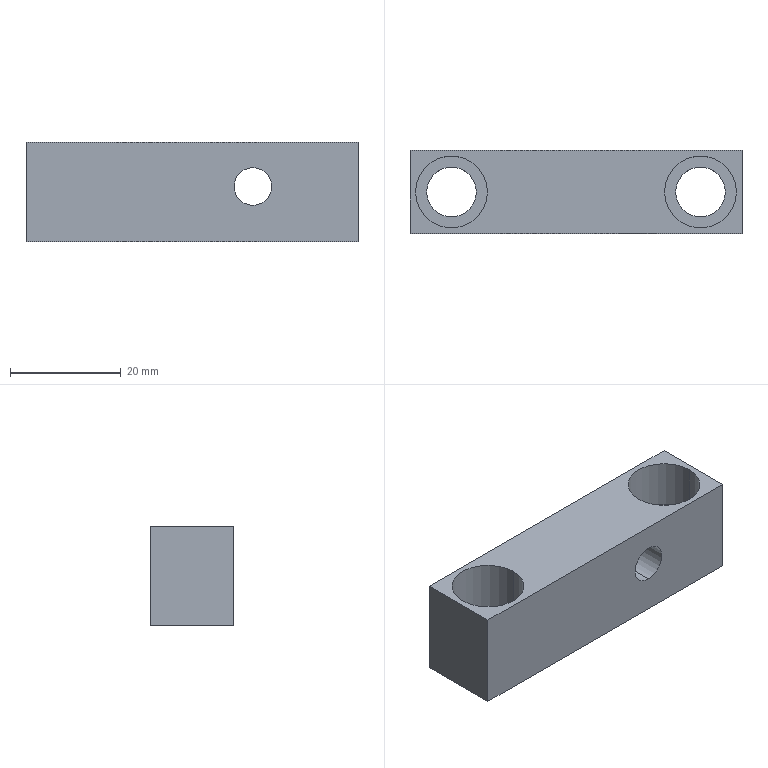Part | STEP file | Tensioning part | 1 solid | 18 faces | box 60 x 15 x 18 mm | volume 12121 mm3 | cylinder 10 | plane 8 | commonest cylinder face diameters 9 x4 13 x4 6.8 x2
STEP:
#1=CARTESIAN_POINT('',(0.,0.,0.));
#2=DIRECTION('',(0.,0.,1.));
#3=DIRECTION('',(1.,0.,0.));
#4=AXIS2_PLACEMENT_3D('',#1,#2,#3);
#5=CARTESIAN_POINT('',(11.,-7.5,13.4));
#6=VERTEX_POINT('',#5);
#7=CARTESIAN_POINT('',(11.,7.5,13.4));
#8=VERTEX_POINT('',#7);
#9=CARTESIAN_POINT('',(11.,7.5,13.4));
#10=DIRECTION('',(0.,1.,0.));
#11=VECTOR('',#10,1.);
#12=LINE('',#9,#11);
#13=CARTESIAN_POINT('',(11.,7.5,10.));
#14=DIRECTION('',(0.,1.,0.));
#15=DIRECTION('',(0.,0.,1.));
#16=AXIS2_PLACEMENT_3D('',#13,#14,#15);
#17=CYLINDRICAL_SURFACE('',#16,3.4);
#18=CARTESIAN_POINT('',(6.283,0.));
#19=DIRECTION('',(0.,1.));
#20=VECTOR('',#19,1.);
#21=LINE('',#18,#20);
#22=(GEOMETRIC_REPRESENTATION_CONTEXT(2)PARAMETRIC_REPRESENTATION_CONTEXT()REPRESENTATION_CONTEXT('',''));
#23=DEFINITIONAL_REPRESENTATION('',(#21),#22);
#24=PCURVE('',#17,#23);
#25=CARTESIAN_POINT('',(11.,7.5,10.));
#26=DIRECTION('',(0.,1.,0.));
#27=DIRECTION('',(0.,0.,1.));
#28=AXIS2_PLACEMENT_3D('',#25,#26,#27);
#29=CYLINDRICAL_SURFACE('',#28,3.4);
#30=CARTESIAN_POINT('',(0.,0.));
#31=DIRECTION('',(0.,1.));
#32=VECTOR('',#31,1.);
#33=LINE('',#30,#32);
#34=(GEOMETRIC_REPRESENTATION_CONTEXT(2)PARAMETRIC_REPRESENTATION_CONTEXT()REPRESENTATION_CONTEXT('',''));
#35=DEFINITIONAL_REPRESENTATION('',(#33),#34);
#36=PCURVE('',#29,#35);
#37=SURFACE_CURVE('',#12,(#24,#36),.PCURVE_S1.);
#38=EDGE_CURVE('',#6,#8,#37,.T.);
#39=ORIENTED_EDGE('',*,*,#38,.T.);
#40=CARTESIAN_POINT('',(11.,7.5,6.6));
#41=VERTEX_POINT('',#40);
#42=CARTESIAN_POINT('',(11.,7.5,10.));
#43=DIRECTION('',(0.,1.,0.));
#44=DIRECTION('',(0.,0.,1.));
#45=AXIS2_PLACEMENT_3D('',#42,#43,#44);
#46=CIRCLE('',#45,3.4);
#47=CARTESIAN_POINT('',(0.,0.));
#48=DIRECTION('',(1.,0.));
#49=VECTOR('',#48,1.);
#50=LINE('',#47,#49);
#51=(GEOMETRIC_REPRESENTATION_CONTEXT(2)PARAMETRIC_REPRESENTATION_CONTEXT()REPRESENTATION_CONTEXT('',''));
#52=DEFINITIONAL_REPRESENTATION('',(#50),#51);
#53=PCURVE('',#17,#52);
#54=CARTESIAN_POINT('',(-30.,7.5,18.));
#55=DIRECTION('',(0.,-1.,0.));
#56=DIRECTION('',(0.,0.,-1.));
#57=AXIS2_PLACEMENT_3D('',#54,#55,#56);
#58=PLANE('',#57);
#59=CARTESIAN_POINT('',(4.6,41.));
#60=CARTESIAN_POINT('',(4.6,46.889));
#61=CARTESIAN_POINT('',(9.7,43.944));
#62=CARTESIAN_POINT('',(14.8,41.));
#63=CARTESIAN_POINT('',(9.7,38.056));
#64=CARTESIAN_POINT('',(4.6,35.111));
#65=CARTESIAN_POINT('',(4.6,41.));
#66=(BOUNDED_CURVE()B_SPLINE_CURVE(2,(#59,#60,#61,#62,#63,#64,#65),.UNSPECIFIED.,.T.,.F.)B_SPLINE_CURVE_WITH_KNOTS((1,2,2,2,2,1),(-2.094,0.,2.094,4.189,6.283,8.378),.UNSPECIFIED.)CURVE()GEOMETRIC_REPRESENTATION_ITEM()RATIONAL_B_SPLINE_CURVE((1.,0.5,1.,0.5,1.,0.5,1.))REPRESENTATION_ITEM(''));
#67=(GEOMETRIC_REPRESENTATION_CONTEXT(2)PARAMETRIC_REPRESENTATION_CONTEXT()REPRESENTATION_CONTEXT('',''));
#68=DEFINITIONAL_REPRESENTATION('',(#66),#67);
#69=PCURVE('',#58,#68);
#70=SURFACE_CURVE('',#46,(#53,#69),.PCURVE_S1.);
#71=EDGE_CURVE('',#41,#8,#70,.T.);
#72=ORIENTED_EDGE('',*,*,#71,.F.);
#73=CARTESIAN_POINT('',(11.,-7.5,6.6));
#74=VERTEX_POINT('',#73);
#75=CARTESIAN_POINT('',(11.,7.5,6.6));
#76=DIRECTION('',(0.,1.,0.));
#77=VECTOR('',#76,1.);
#78=LINE('',#75,#77);
#79=CARTESIAN_POINT('',(3.142,0.));
#80=DIRECTION('',(0.,1.));
#81=VECTOR('',#80,1.);
#82=LINE('',#79,#81);
#83=(GEOMETRIC_REPRESENTATION_CONTEXT(2)PARAMETRIC_REPRESENTATION_CONTEXT()REPRESENTATION_CONTEXT('',''));
#84=DEFINITIONAL_REPRESENTATION('',(#82),#83);
#85=PCURVE('',#17,#84);
#86=CARTESIAN_POINT('',(3.142,0.));
#87=DIRECTION('',(0.,1.));
#88=VECTOR('',#87,1.);
#89=LINE('',#86,#88);
#90=(GEOMETRIC_REPRESENTATION_CONTEXT(2)PARAMETRIC_REPRESENTATION_CONTEXT()REPRESENTATION_CONTEXT('',''));
#91=DEFINITIONAL_REPRESENTATION('',(#89),#90);
#92=PCURVE('',#29,#91);
#93=SURFACE_CURVE('',#78,(#85,#92),.PCURVE_S1.);
#94=EDGE_CURVE('',#74,#41,#93,.T.);
#95=ORIENTED_EDGE('',*,*,#94,.F.);
#96=CARTESIAN_POINT('',(11.,-7.5,10.));
#97=DIRECTION('',(0.,1.,0.));
#98=DIRECTION('',(0.,0.,1.));
#99=AXIS2_PLACEMENT_3D('',#96,#97,#98);
#100=CIRCLE('',#99,3.4);
#101=CARTESIAN_POINT('',(0.,-15.));
#102=DIRECTION('',(1.,0.));
#103=VECTOR('',#102,1.);
#104=LINE('',#101,#103);
#105=(GEOMETRIC_REPRESENTATION_CONTEXT(2)PARAMETRIC_REPRESENTATION_CONTEXT()REPRESENTATION_CONTEXT('',''));
#106=DEFINITIONAL_REPRESENTATION('',(#104),#105);
#107=PCURVE('',#17,#106);
#108=CARTESIAN_POINT('',(-30.,-7.5,18.));
#109=DIRECTION('',(0.,1.,0.));
#110=DIRECTION('',(0.,0.,1.));
#111=AXIS2_PLACEMENT_3D('',#108,#109,#110);
#112=PLANE('',#111);
#113=CARTESIAN_POINT('',(-8.,41.));
#114=DIRECTION('',(1.,0.));
#115=AXIS2_PLACEMENT_2D('',#113,#114);
#116=CIRCLE('',#115,3.4);
#117=(GEOMETRIC_REPRESENTATION_CONTEXT(2)PARAMETRIC_REPRESENTATION_CONTEXT()REPRESENTATION_CONTEXT('',''));
#118=DEFINITIONAL_REPRESENTATION('',(#116),#117);
#119=PCURVE('',#112,#118);
#120=SURFACE_CURVE('',#100,(#107,#119),.PCURVE_S1.);
#121=EDGE_CURVE('',#74,#6,#120,.T.);
#122=ORIENTED_EDGE('',*,*,#121,.T.);
#123=EDGE_LOOP('',(#39,#72,#95,#122));
#124=FACE_BOUND('',#123,.F.);
#125=ADVANCED_FACE('',(#124),#17,.F.);
#126=CARTESIAN_POINT('',(-16.,0.,9.));
#127=VERTEX_POINT('',#126);
#128=CARTESIAN_POINT('',(-16.,0.,18.));
#129=VERTEX_POINT('',#128);
#130=CARTESIAN_POINT('',(-16.,0.,18.));
#131=DIRECTION('',(0.,0.,1.));
#132=VECTOR('',#131,1.);
#133=LINE('',#130,#132);
#134=CARTESIAN_POINT('',(-22.5,0.,18.));
#135=DIRECTION('',(0.,0.,1.));
#136=DIRECTION('',(1.,0.,0.));
#137=AXIS2_PLACEMENT_3D('',#134,#135,#136);
#138=CYLINDRICAL_SURFACE('',#137,6.5);
#139=CARTESIAN_POINT('',(6.283,0.));
#140=DIRECTION('',(0.,1.));
#141=VECTOR('',#140,1.);
#142=LINE('',#139,#141);
#143=(GEOMETRIC_REPRESENTATION_CONTEXT(2)PARAMETRIC_REPRESENTATION_CONTEXT()REPRESENTATION_CONTEXT('',''));
#144=DEFINITIONAL_REPRESENTATION('',(#142),#143);
#145=PCURVE('',#138,#144);
#146=CARTESIAN_POINT('',(-22.5,0.,18.));
#147=DIRECTION('',(0.,0.,1.));
#148=DIRECTION('',(1.,0.,0.));
#149=AXIS2_PLACEMENT_3D('',#146,#147,#148);
#150=CYLINDRICAL_SURFACE('',#149,6.5);
#151=CARTESIAN_POINT('',(0.,0.));
#152=DIRECTION('',(0.,1.));
#153=VECTOR('',#152,1.);
#154=LINE('',#151,#153);
#155=(GEOMETRIC_REPRESENTATION_CONTEXT(2)PARAMETRIC_REPRESENTATION_CONTEXT()REPRESENTATION_CONTEXT('',''));
#156=DEFINITIONAL_REPRESENTATION('',(#154),#155);
#157=PCURVE('',#150,#156);
#158=SURFACE_CURVE('',#133,(#145,#157),.PCURVE_S1.);
#159=EDGE_CURVE('',#127,#129,#158,.T.);
#160=ORIENTED_EDGE('',*,*,#159,.T.);
#161=CARTESIAN_POINT('',(-29.,0.,18.));
#162=VERTEX_POINT('',#161);
#163=CARTESIAN_POINT('',(-22.5,0.,18.));
#164=DIRECTION('',(0.,0.,1.));
#165=DIRECTION('',(1.,0.,0.));
#166=AXIS2_PLACEMENT_3D('',#163,#164,#165);
#167=CIRCLE('',#166,6.5);
#168=CARTESIAN_POINT('',(0.,0.));
#169=DIRECTION('',(1.,0.));
#170=VECTOR('',#169,1.);
#171=LINE('',#168,#170);
#172=(GEOMETRIC_REPRESENTATION_CONTEXT(2)PARAMETRIC_REPRESENTATION_CONTEXT()REPRESENTATION_CONTEXT('',''));
#173=DEFINITIONAL_REPRESENTATION('',(#171),#172);
#174=PCURVE('',#138,#173);
#175=CARTESIAN_POINT('',(0.,0.,18.));
#176=DIRECTION('',(0.,0.,1.));
#177=DIRECTION('',(1.,0.,0.));
#178=AXIS2_PLACEMENT_3D('',#175,#176,#177);
#179=PLANE('',#178);
#180=CARTESIAN_POINT('',(-22.5,0.));
#181=DIRECTION('',(1.,0.));
#182=AXIS2_PLACEMENT_2D('',#180,#181);
#183=CIRCLE('',#182,6.5);
#184=(GEOMETRIC_REPRESENTATION_CONTEXT(2)PARAMETRIC_REPRESENTATION_CONTEXT()REPRESENTATION_CONTEXT('',''));
#185=DEFINITIONAL_REPRESENTATION('',(#183),#184);
#186=PCURVE('',#179,#185);
#187=SURFACE_CURVE('',#167,(#174,#186),.PCURVE_S1.);
#188=EDGE_CURVE('',#162,#129,#187,.T.);
#189=ORIENTED_EDGE('',*,*,#188,.F.);
#190=CARTESIAN_POINT('',(-29.,0.,9.));
#191=VERTEX_POINT('',#190);
#192=CARTESIAN_POINT('',(-29.,0.,18.));
#193=DIRECTION('',(0.,0.,1.));
#194=VECTOR('',#193,1.);
#195=LINE('',#192,#194);
#196=CARTESIAN_POINT('',(3.142,0.));
#197=DIRECTION('',(0.,1.));
#198=VECTOR('',#197,1.);
#199=LINE('',#196,#198);
#200=(GEOMETRIC_REPRESENTATION_CONTEXT(2)PARAMETRIC_REPRESENTATION_CONTEXT()REPRESENTATION_CONTEXT('',''));
#201=DEFINITIONAL_REPRESENTATION('',(#199),#200);
#202=PCURVE('',#138,#201);
#203=CARTESIAN_POINT('',(3.142,0.));
#204=DIRECTION('',(0.,1.));
#205=VECTOR('',#204,1.);
#206=LINE('',#203,#205);
#207=(GEOMETRIC_REPRESENTATION_CONTEXT(2)PARAMETRIC_REPRESENTATION_CONTEXT()REPRESENTATION_CONTEXT('',''));
#208=DEFINITIONAL_REPRESENTATION('',(#206),#207);
#209=PCURVE('',#150,#208);
#210=SURFACE_CURVE('',#195,(#202,#209),.PCURVE_S1.);
#211=EDGE_CURVE('',#191,#162,#210,.T.);
#212=ORIENTED_EDGE('',*,*,#211,.F.);
#213=CARTESIAN_POINT('',(-22.5,0.,9.));
#214=DIRECTION('',(0.,0.,1.));
#215=DIRECTION('',(1.,0.,0.));
#216=AXIS2_PLACEMENT_3D('',#213,#214,#215);
#217=CIRCLE('',#216,6.5);
#218=CARTESIAN_POINT('',(0.,-9.));
#219=DIRECTION('',(1.,0.));
#220=VECTOR('',#219,1.);
#221=LINE('',#218,#220);
#222=(GEOMETRIC_REPRESENTATION_CONTEXT(2)PARAMETRIC_REPRESENTATION_CONTEXT()REPRESENTATION_CONTEXT('',''));
#223=DEFINITIONAL_REPRESENTATION('',(#221),#222);
#224=PCURVE('',#138,#223);
#225=CARTESIAN_POINT('',(-18.,0.,9.));
#226=DIRECTION('',(0.,0.,-1.));
#227=DIRECTION('',(-1.,0.,0.));
#228=AXIS2_PLACEMENT_3D('',#225,#226,#227);
#229=PLANE('',#228);
#230=CARTESIAN_POINT('',(-2.,0.));
#231=CARTESIAN_POINT('',(-2.,11.258));
#232=CARTESIAN_POINT('',(7.75,5.629));
#233=CARTESIAN_POINT('',(17.5,0.));
#234=CARTESIAN_POINT('',(7.75,-5.629));
#235=CARTESIAN_POINT('',(-2.,-11.258));
#236=CARTESIAN_POINT('',(-2.,0.));
#237=(BOUNDED_CURVE()B_SPLINE_CURVE(2,(#230,#231,#232,#233,#234,#235,#236),.UNSPECIFIED.,.T.,.F.)B_SPLINE_CURVE_WITH_KNOTS((1,2,2,2,2,1),(-2.094,0.,2.094,4.189,6.283,8.378),.UNSPECIFIED.)CURVE()GEOMETRIC_REPRESENTATION_ITEM()RATIONAL_B_SPLINE_CURVE((1.,0.5,1.,0.5,1.,0.5,1.))REPRESENTATION_ITEM(''));
#238=(GEOMETRIC_REPRESENTATION_CONTEXT(2)PARAMETRIC_REPRESENTATION_CONTEXT()REPRESENTATION_CONTEXT('',''));
#239=DEFINITIONAL_REPRESENTATION('',(#237),#238);
#240=PCURVE('',#229,#239);
#241=SURFACE_CURVE('',#217,(#224,#240),.PCURVE_S1.);
#242=EDGE_CURVE('',#191,#127,#241,.T.);
#243=ORIENTED_EDGE('',*,*,#242,.T.);
#244=EDGE_LOOP('',(#160,#189,#212,#243));
#245=FACE_BOUND('',#244,.F.);
#246=ADVANCED_FACE('',(#245),#138,.F.);
#247=CARTESIAN_POINT('',(-18.,0.,0.));
#248=VERTEX_POINT('',#247);
#249=CARTESIAN_POINT('',(-18.,0.,9.));
#250=VERTEX_POINT('',#249);
#251=CARTESIAN_POINT('',(-18.,0.,18.));
#252=DIRECTION('',(0.,0.,1.));
#253=VECTOR('',#252,1.);
#254=LINE('',#251,#253);
#255=CARTESIAN_POINT('',(-22.5,0.,18.));
#256=DIRECTION('',(0.,0.,1.));
#257=DIRECTION('',(1.,0.,0.));
#258=AXIS2_PLACEMENT_3D('',#255,#256,#257);
#259=CYLINDRICAL_SURFACE('',#258,4.5);
#260=CARTESIAN_POINT('',(6.283,0.));
#261=DIRECTION('',(0.,1.));
#262=VECTOR('',#261,1.);
#263=LINE('',#260,#262);
#264=(GEOMETRIC_REPRESENTATION_CONTEXT(2)PARAMETRIC_REPRESENTATION_CONTEXT()REPRESENTATION_CONTEXT('',''));
#265=DEFINITIONAL_REPRESENTATION('',(#263),#264);
#266=PCURVE('',#259,#265);
#267=CARTESIAN_POINT('',(-22.5,0.,18.));
#268=DIRECTION('',(0.,0.,1.));
#269=DIRECTION('',(1.,0.,0.));
#270=AXIS2_PLACEMENT_3D('',#267,#268,#269);
#271=CYLINDRICAL_SURFACE('',#270,4.5);
#272=CARTESIAN_POINT('',(0.,0.));
#273=DIRECTION('',(0.,1.));
#274=VECTOR('',#273,1.);
#275=LINE('',#272,#274);
#276=(GEOMETRIC_REPRESENTATION_CONTEXT(2)PARAMETRIC_REPRESENTATION_CONTEXT()REPRESENTATION_CONTEXT('',''));
#277=DEFINITIONAL_REPRESENTATION('',(#275),#276);
#278=PCURVE('',#271,#277);
#279=SURFACE_CURVE('',#254,(#266,#278),.PCURVE_S1.);
#280=EDGE_CURVE('',#248,#250,#279,.T.);
#281=ORIENTED_EDGE('',*,*,#280,.T.);
#282=CARTESIAN_POINT('',(-27.,0.,9.));
#283=VERTEX_POINT('',#282);
#284=CARTESIAN_POINT('',(-22.5,0.,9.));
#285=DIRECTION('',(0.,0.,1.));
#286=DIRECTION('',(1.,0.,0.));
#287=AXIS2_PLACEMENT_3D('',#284,#285,#286);
#288=CIRCLE('',#287,4.5);
#289=CARTESIAN_POINT('',(0.,-9.));
#290=DIRECTION('',(1.,0.));
#291=VECTOR('',#290,1.);
#292=LINE('',#289,#291);
#293=(GEOMETRIC_REPRESENTATION_CONTEXT(2)PARAMETRIC_REPRESENTATION_CONTEXT()REPRESENTATION_CONTEXT('',''));
#294=DEFINITIONAL_REPRESENTATION('',(#292),#293);
#295=PCURVE('',#259,#294);
#296=CARTESIAN_POINT('',(0.,0.));
#297=CARTESIAN_POINT('',(0.,7.794));
#298=CARTESIAN_POINT('',(6.75,3.897));
#299=CARTESIAN_POINT('',(13.5,0.));
#300=CARTESIAN_POINT('',(6.75,-3.897));
#301=CARTESIAN_POINT('',(0.,-7.794));
#302=CARTESIAN_POINT('',(0.,0.));
#303=(BOUNDED_CURVE()B_SPLINE_CURVE(2,(#296,#297,#298,#299,#300,#301,#302),.UNSPECIFIED.,.T.,.F.)B_SPLINE_CURVE_WITH_KNOTS((1,2,2,2,2,1),(-2.094,0.,2.094,4.189,6.283,8.378),.UNSPECIFIED.)CURVE()GEOMETRIC_REPRESENTATION_ITEM()RATIONAL_B_SPLINE_CURVE((1.,0.5,1.,0.5,1.,0.5,1.))REPRESENTATION_ITEM(''));
#304=(GEOMETRIC_REPRESENTATION_CONTEXT(2)PARAMETRIC_REPRESENTATION_CONTEXT()REPRESENTATION_CONTEXT('',''));
#305=DEFINITIONAL_REPRESENTATION('',(#303),#304);
#306=PCURVE('',#229,#305);
#307=SURFACE_CURVE('',#288,(#295,#306),.PCURVE_S1.);
#308=EDGE_CURVE('',#283,#250,#307,.T.);
#309=ORIENTED_EDGE('',*,*,#308,.F.);
#310=CARTESIAN_POINT('',(-27.,0.,0.));
#311=VERTEX_POINT('',#310);
#312=CARTESIAN_POINT('',(-27.,0.,18.));
#313=DIRECTION('',(0.,0.,1.));
#314=VECTOR('',#313,1.);
#315=LINE('',#312,#314);
#316=CARTESIAN_POINT('',(3.142,0.));
#317=DIRECTION('',(0.,1.));
#318=VECTOR('',#317,1.);
#319=LINE('',#316,#318);
#320=(GEOMETRIC_REPRESENTATION_CONTEXT(2)PARAMETRIC_REPRESENTATION_CONTEXT()REPRESENTATION_CONTEXT('',''));
#321=DEFINITIONAL_REPRESENTATION('',(#319),#320);
#322=PCURVE('',#259,#321);
#323=CARTESIAN_POINT('',(3.142,0.));
#324=DIRECTION('',(0.,1.));
#325=VECTOR('',#324,1.);
#326=LINE('',#323,#325);
#327=(GEOMETRIC_REPRESENTATION_CONTEXT(2)PARAMETRIC_REPRESENTATION_CONTEXT()REPRESENTATION_CONTEXT('',''));
#328=DEFINITIONAL_REPRESENTATION('',(#326),#327);
#329=PCURVE('',#271,#328);
#330=SURFACE_CURVE('',#315,(#322,#329),.PCURVE_S1.);
#331=EDGE_CURVE('',#311,#283,#330,.T.);
#332=ORIENTED_EDGE('',*,*,#331,.F.);
#333=CARTESIAN_POINT('',(-22.5,0.,0.));
#334=DIRECTION('',(0.,0.,1.));
#335=DIRECTION('',(1.,0.,0.));
#336=AXIS2_PLACEMENT_3D('',#333,#334,#335);
#337=CIRCLE('',#336,4.5);
#338=CARTESIAN_POINT('',(0.,-18.));
#339=DIRECTION('',(1.,0.));
#340=VECTOR('',#339,1.);
#341=LINE('',#338,#340);
#342=(GEOMETRIC_REPRESENTATION_CONTEXT(2)PARAMETRIC_REPRESENTATION_CONTEXT()REPRESENTATION_CONTEXT('',''));
#343=DEFINITIONAL_REPRESENTATION('',(#341),#342);
#344=PCURVE('',#259,#343);
#345=CARTESIAN_POINT('',(0.,0.,0.));
#346=DIRECTION('',(0.,0.,1.));
#347=DIRECTION('',(1.,0.,0.));
#348=AXIS2_PLACEMENT_3D('',#345,#346,#347);
#349=PLANE('',#348);
#350=CARTESIAN_POINT('',(-22.5,0.));
#351=DIRECTION('',(1.,0.));
#352=AXIS2_PLACEMENT_2D('',#350,#351);
#353=CIRCLE('',#352,4.5);
#354=(GEOMETRIC_REPRESENTATION_CONTEXT(2)PARAMETRIC_REPRESENTATION_CONTEXT()REPRESENTATION_CONTEXT('',''));
#355=DEFINITIONAL_REPRESENTATION('',(#353),#354);
#356=PCURVE('',#349,#355);
#357=SURFACE_CURVE('',#337,(#344,#356),.PCURVE_S1.);
#358=EDGE_CURVE('',#311,#248,#357,.T.);
#359=ORIENTED_EDGE('',*,*,#358,.T.);
#360=EDGE_LOOP('',(#281,#309,#332,#359));
#361=FACE_BOUND('',#360,.F.);
#362=ADVANCED_FACE('',(#361),#259,.F.);
#363=CARTESIAN_POINT('',(29.,0.,9.));
#364=VERTEX_POINT('',#363);
#365=CARTESIAN_POINT('',(29.,0.,18.));
#366=VERTEX_POINT('',#365);
#367=CARTESIAN_POINT('',(29.,0.,18.));
#368=DIRECTION('',(0.,0.,1.));
#369=VECTOR('',#368,1.);
#370=LINE('',#367,#369);
#371=CARTESIAN_POINT('',(22.5,0.,18.));
#372=DIRECTION('',(0.,0.,1.));
#373=DIRECTION('',(1.,0.,0.));
#374=AXIS2_PLACEMENT_3D('',#371,#372,#373);
#375=CYLINDRICAL_SURFACE('',#374,6.5);
#376=CARTESIAN_POINT('',(6.283,0.));
#377=DIRECTION('',(0.,1.));
#378=VECTOR('',#377,1.);
#379=LINE('',#376,#378);
#380=(GEOMETRIC_REPRESENTATION_CONTEXT(2)PARAMETRIC_REPRESENTATION_CONTEXT()REPRESENTATION_CONTEXT('',''));
#381=DEFINITIONAL_REPRESENTATION('',(#379),#380);
#382=PCURVE('',#375,#381);
#383=CARTESIAN_POINT('',(22.5,0.,18.));
#384=DIRECTION('',(0.,0.,1.));
#385=DIRECTION('',(1.,0.,0.));
#386=AXIS2_PLACEMENT_3D('',#383,#384,#385);
#387=CYLINDRICAL_SURFACE('',#386,6.5);
#388=CARTESIAN_POINT('',(0.,0.));
#389=DIRECTION('',(0.,1.));
#390=VECTOR('',#389,1.);
#391=LINE('',#388,#390);
#392=(GEOMETRIC_REPRESENTATION_CONTEXT(2)PARAMETRIC_REPRESENTATION_CONTEXT()REPRESENTATION_CONTEXT('',''));
#393=DEFINITIONAL_REPRESENTATION('',(#391),#392);
#394=PCURVE('',#387,#393);
#395=SURFACE_CURVE('',#370,(#382,#394),.PCURVE_S1.);
#396=EDGE_CURVE('',#364,#366,#395,.T.);
#397=ORIENTED_EDGE('',*,*,#396,.T.);
#398=CARTESIAN_POINT('',(16.,0.,18.));
#399=VERTEX_POINT('',#398);
#400=CARTESIAN_POINT('',(22.5,0.,18.));
#401=DIRECTION('',(0.,0.,1.));
#402=DIRECTION('',(1.,0.,0.));
#403=AXIS2_PLACEMENT_3D('',#400,#401,#402);
#404=CIRCLE('',#403,6.5);
#405=CARTESIAN_POINT('',(0.,0.));
#406=DIRECTION('',(1.,0.));
#407=VECTOR('',#406,1.);
#408=LINE('',#405,#407);
#409=(GEOMETRIC_REPRESENTATION_CONTEXT(2)PARAMETRIC_REPRESENTATION_CONTEXT()REPRESENTATION_CONTEXT('',''));
#410=DEFINITIONAL_REPRESENTATION('',(#408),#409);
#411=PCURVE('',#375,#410);
#412=CARTESIAN_POINT('',(22.5,0.));
#413=DIRECTION('',(1.,0.));
#414=AXIS2_PLACEMENT_2D('',#412,#413);
#415=CIRCLE('',#414,6.5);
#416=(GEOMETRIC_REPRESENTATION_CONTEXT(2)PARAMETRIC_REPRESENTATION_CONTEXT()REPRESENTATION_CONTEXT('',''));
#417=DEFINITIONAL_REPRESENTATION('',(#415),#416);
#418=PCURVE('',#179,#417);
#419=SURFACE_CURVE('',#404,(#411,#418),.PCURVE_S1.);
#420=EDGE_CURVE('',#399,#366,#419,.T.);
#421=ORIENTED_EDGE('',*,*,#420,.F.);
#422=CARTESIAN_POINT('',(16.,0.,9.));
#423=VERTEX_POINT('',#422);
#424=CARTESIAN_POINT('',(16.,0.,18.));
#425=DIRECTION('',(0.,0.,1.));
#426=VECTOR('',#425,1.);
#427=LINE('',#424,#426);
#428=CARTESIAN_POINT('',(3.142,0.));
#429=DIRECTION('',(0.,1.));
#430=VECTOR('',#429,1.);
#431=LINE('',#428,#430);
#432=(GEOMETRIC_REPRESENTATION_CONTEXT(2)PARAMETRIC_REPRESENTATION_CONTEXT()REPRESENTATION_CONTEXT('',''));
#433=DEFINITIONAL_REPRESENTATION('',(#431),#432);
#434=PCURVE('',#375,#433);
#435=CARTESIAN_POINT('',(3.142,0.));
#436=DIRECTION('',(0.,1.));
#437=VECTOR('',#436,1.);
#438=LINE('',#435,#437);
#439=(GEOMETRIC_REPRESENTATION_CONTEXT(2)PARAMETRIC_REPRESENTATION_CONTEXT()REPRESENTATION_CONTEXT('',''));
#440=DEFINITIONAL_REPRESENTATION('',(#438),#439);
#441=PCURVE('',#387,#440);
#442=SURFACE_CURVE('',#427,(#434,#441),.PCURVE_S1.);
#443=EDGE_CURVE('',#423,#399,#442,.T.);
#444=ORIENTED_EDGE('',*,*,#443,.F.);
#445=CARTESIAN_POINT('',(22.5,0.,9.));
#446=DIRECTION('',(0.,0.,1.));
#447=DIRECTION('',(1.,0.,0.));
#448=AXIS2_PLACEMENT_3D('',#445,#446,#447);
#449=CIRCLE('',#448,6.5);
#450=CARTESIAN_POINT('',(0.,-9.));
#451=DIRECTION('',(1.,0.));
#452=VECTOR('',#451,1.);
#453=LINE('',#450,#452);
#454=(GEOMETRIC_REPRESENTATION_CONTEXT(2)PARAMETRIC_REPRESENTATION_CONTEXT()REPRESENTATION_CONTEXT('',''));
#455=DEFINITIONAL_REPRESENTATION('',(#453),#454);
#456=PCURVE('',#375,#455);
#457=CARTESIAN_POINT('',(27.,0.,9.));
#458=DIRECTION('',(0.,0.,-1.));
#459=DIRECTION('',(-1.,0.,0.));
#460=AXIS2_PLACEMENT_3D('',#457,#458,#459);
#461=PLANE('',#460);
#462=CARTESIAN_POINT('',(-2.,0.));
#463=CARTESIAN_POINT('',(-2.,11.258));
#464=CARTESIAN_POINT('',(7.75,5.629));
#465=CARTESIAN_POINT('',(17.5,0.));
#466=CARTESIAN_POINT('',(7.75,-5.629));
#467=CARTESIAN_POINT('',(-2.,-11.258));
#468=CARTESIAN_POINT('',(-2.,0.));
#469=(BOUNDED_CURVE()B_SPLINE_CURVE(2,(#462,#463,#464,#465,#466,#467,#468),.UNSPECIFIED.,.T.,.F.)B_SPLINE_CURVE_WITH_KNOTS((1,2,2,2,2,1),(-2.094,0.,2.094,4.189,6.283,8.378),.UNSPECIFIED.)CURVE()GEOMETRIC_REPRESENTATION_ITEM()RATIONAL_B_SPLINE_CURVE((1.,0.5,1.,0.5,1.,0.5,1.))REPRESENTATION_ITEM(''));
#470=(GEOMETRIC_REPRESENTATION_CONTEXT(2)PARAMETRIC_REPRESENTATION_CONTEXT()REPRESENTATION_CONTEXT('',''));
#471=DEFINITIONAL_REPRESENTATION('',(#469),#470);
#472=PCURVE('',#461,#471);
#473=SURFACE_CURVE('',#449,(#456,#472),.PCURVE_S1.);
#474=EDGE_CURVE('',#423,#364,#473,.T.);
#475=ORIENTED_EDGE('',*,*,#474,.T.);
#476=EDGE_LOOP('',(#397,#421,#444,#475));
#477=FACE_BOUND('',#476,.F.);
#478=ADVANCED_FACE('',(#477),#375,.F.);
#479=CARTESIAN_POINT('',(27.,0.,0.));
#480=VERTEX_POINT('',#479);
#481=CARTESIAN_POINT('',(27.,0.,9.));
#482=VERTEX_POINT('',#481);
#483=CARTESIAN_POINT('',(27.,0.,18.));
#484=DIRECTION('',(0.,0.,1.));
#485=VECTOR('',#484,1.);
#486=LINE('',#483,#485);
#487=CARTESIAN_POINT('',(22.5,0.,18.));
#488=DIRECTION('',(0.,0.,1.));
#489=DIRECTION('',(1.,0.,0.));
#490=AXIS2_PLACEMENT_3D('',#487,#488,#489);
#491=CYLINDRICAL_SURFACE('',#490,4.5);
#492=CARTESIAN_POINT('',(6.283,0.));
#493=DIRECTION('',(0.,1.));
#494=VECTOR('',#493,1.);
#495=LINE('',#492,#494);
#496=(GEOMETRIC_REPRESENTATION_CONTEXT(2)PARAMETRIC_REPRESENTATION_CONTEXT()REPRESENTATION_CONTEXT('',''));
#497=DEFINITIONAL_REPRESENTATION('',(#495),#496);
#498=PCURVE('',#491,#497);
#499=CARTESIAN_POINT('',(22.5,0.,18.));
#500=DIRECTION('',(0.,0.,1.));
#501=DIRECTION('',(1.,0.,0.));
#502=AXIS2_PLACEMENT_3D('',#499,#500,#501);
#503=CYLINDRICAL_SURFACE('',#502,4.5);
#504=CARTESIAN_POINT('',(0.,0.));
#505=DIRECTION('',(0.,1.));
#506=VECTOR('',#505,1.);
#507=LINE('',#504,#506);
#508=(GEOMETRIC_REPRESENTATION_CONTEXT(2)PARAMETRIC_REPRESENTATION_CONTEXT()REPRESENTATION_CONTEXT('',''));
#509=DEFINITIONAL_REPRESENTATION('',(#507),#508);
#510=PCURVE('',#503,#509);
#511=SURFACE_CURVE('',#486,(#498,#510),.PCURVE_S1.);
#512=EDGE_CURVE('',#480,#482,#511,.T.);
#513=ORIENTED_EDGE('',*,*,#512,.T.);
#514=CARTESIAN_POINT('',(18.,0.,9.));
#515=VERTEX_POINT('',#514);
#516=CARTESIAN_POINT('',(22.5,0.,9.));
#517=DIRECTION('',(0.,0.,1.));
#518=DIRECTION('',(1.,0.,0.));
#519=AXIS2_PLACEMENT_3D('',#516,#517,#518);
#520=CIRCLE('',#519,4.5);
#521=CARTESIAN_POINT('',(0.,-9.));
#522=DIRECTION('',(1.,0.));
#523=VECTOR('',#522,1.);
#524=LINE('',#521,#523);
#525=(GEOMETRIC_REPRESENTATION_CONTEXT(2)PARAMETRIC_REPRESENTATION_CONTEXT()REPRESENTATION_CONTEXT('',''));
#526=DEFINITIONAL_REPRESENTATION('',(#524),#525);
#527=PCURVE('',#491,#526);
#528=CARTESIAN_POINT('',(0.,0.));
#529=CARTESIAN_POINT('',(0.,7.794));
#530=CARTESIAN_POINT('',(6.75,3.897));
#531=CARTESIAN_POINT('',(13.5,0.));
#532=CARTESIAN_POINT('',(6.75,-3.897));
#533=CARTESIAN_POINT('',(0.,-7.794));
#534=CARTESIAN_POINT('',(0.,0.));
#535=(BOUNDED_CURVE()B_SPLINE_CURVE(2,(#528,#529,#530,#531,#532,#533,#534),.UNSPECIFIED.,.T.,.F.)B_SPLINE_CURVE_WITH_KNOTS((1,2,2,2,2,1),(-2.094,0.,2.094,4.189,6.283,8.378),.UNSPECIFIED.)CURVE()GEOMETRIC_REPRESENTATION_ITEM()RATIONAL_B_SPLINE_CURVE((1.,0.5,1.,0.5,1.,0.5,1.))REPRESENTATION_ITEM(''));
#536=(GEOMETRIC_REPRESENTATION_CONTEXT(2)PARAMETRIC_REPRESENTATION_CONTEXT()REPRESENTATION_CONTEXT('',''));
#537=DEFINITIONAL_REPRESENTATION('',(#535),#536);
#538=PCURVE('',#461,#537);
#539=SURFACE_CURVE('',#520,(#527,#538),.PCURVE_S1.);
#540=EDGE_CURVE('',#515,#482,#539,.T.);
#541=ORIENTED_EDGE('',*,*,#540,.F.);
#542=CARTESIAN_POINT('',(18.,0.,0.));
#543=VERTEX_POINT('',#542);
#544=CARTESIAN_POINT('',(18.,0.,18.));
#545=DIRECTION('',(0.,0.,1.));
#546=VECTOR('',#545,1.);
#547=LINE('',#544,#546);
#548=CARTESIAN_POINT('',(3.142,0.));
#549=DIRECTION('',(0.,1.));
#550=VECTOR('',#549,1.);
#551=LINE('',#548,#550);
#552=(GEOMETRIC_REPRESENTATION_CONTEXT(2)PARAMETRIC_REPRESENTATION_CONTEXT()REPRESENTATION_CONTEXT('',''));
#553=DEFINITIONAL_REPRESENTATION('',(#551),#552);
#554=PCURVE('',#491,#553);
#555=CARTESIAN_POINT('',(3.142,0.));
#556=DIRECTION('',(0.,1.));
#557=VECTOR('',#556,1.);
#558=LINE('',#555,#557);
#559=(GEOMETRIC_REPRESENTATION_CONTEXT(2)PARAMETRIC_REPRESENTATION_CONTEXT()REPRESENTATION_CONTEXT('',''));
#560=DEFINITIONAL_REPRESENTATION('',(#558),#559);
#561=PCURVE('',#503,#560);
#562=SURFACE_CURVE('',#547,(#554,#561),.PCURVE_S1.);
#563=EDGE_CURVE('',#543,#515,#562,.T.);
#564=ORIENTED_EDGE('',*,*,#563,.F.);
#565=CARTESIAN_POINT('',(22.5,0.,0.));
#566=DIRECTION('',(0.,0.,1.));
#567=DIRECTION('',(1.,0.,0.));
#568=AXIS2_PLACEMENT_3D('',#565,#566,#567);
#569=CIRCLE('',#568,4.5);
#570=CARTESIAN_POINT('',(0.,-18.));
#571=DIRECTION('',(1.,0.));
#572=VECTOR('',#571,1.);
#573=LINE('',#570,#572);
#574=(GEOMETRIC_REPRESENTATION_CONTEXT(2)PARAMETRIC_REPRESENTATION_CONTEXT()REPRESENTATION_CONTEXT('',''));
#575=DEFINITIONAL_REPRESENTATION('',(#573),#574);
#576=PCURVE('',#491,#575);
#577=CARTESIAN_POINT('',(22.5,0.));
#578=DIRECTION('',(1.,0.));
#579=AXIS2_PLACEMENT_2D('',#577,#578);
#580=CIRCLE('',#579,4.5);
#581=(GEOMETRIC_REPRESENTATION_CONTEXT(2)PARAMETRIC_REPRESENTATION_CONTEXT()REPRESENTATION_CONTEXT('',''));
#582=DEFINITIONAL_REPRESENTATION('',(#580),#581);
#583=PCURVE('',#349,#582);
#584=SURFACE_CURVE('',#569,(#576,#583),.PCURVE_S1.);
#585=EDGE_CURVE('',#543,#480,#584,.T.);
#586=ORIENTED_EDGE('',*,*,#585,.T.);
#587=EDGE_LOOP('',(#513,#541,#564,#586));
#588=FACE_BOUND('',#587,.F.);
#589=ADVANCED_FACE('',(#588),#491,.F.);
#590=CARTESIAN_POINT('',(30.,-7.5,0.));
#591=VERTEX_POINT('',#590);
#592=CARTESIAN_POINT('',(30.,7.5,0.));
#593=VERTEX_POINT('',#592);
#594=CARTESIAN_POINT('',(30.,7.5,0.));
#595=DIRECTION('',(0.,1.,0.));
#596=VECTOR('',#595,1.);
#597=LINE('',#594,#596);
#598=CARTESIAN_POINT('',(30.,7.5,18.));
#599=DIRECTION('',(-1.,0.,0.));
#600=DIRECTION('',(0.,-1.,0.));
#601=AXIS2_PLACEMENT_3D('',#598,#599,#600);
#602=PLANE('',#601);
#603=CARTESIAN_POINT('',(0.,-18.));
#604=DIRECTION('',(-1.,0.));
#605=VECTOR('',#604,1.);
#606=LINE('',#603,#605);
#607=(GEOMETRIC_REPRESENTATION_CONTEXT(2)PARAMETRIC_REPRESENTATION_CONTEXT()REPRESENTATION_CONTEXT('',''));
#608=DEFINITIONAL_REPRESENTATION('',(#606),#607);
#609=PCURVE('',#602,#608);
#610=CARTESIAN_POINT('',(30.,7.5));
#611=DIRECTION('',(0.,1.));
#612=VECTOR('',#611,1.);
#613=LINE('',#610,#612);
#614=(GEOMETRIC_REPRESENTATION_CONTEXT(2)PARAMETRIC_REPRESENTATION_CONTEXT()REPRESENTATION_CONTEXT('',''));
#615=DEFINITIONAL_REPRESENTATION('',(#613),#614);
#616=PCURVE('',#349,#615);
#617=SURFACE_CURVE('',#597,(#609,#616),.PCURVE_S1.);
#618=EDGE_CURVE('',#591,#593,#617,.T.);
#619=ORIENTED_EDGE('',*,*,#618,.T.);
#620=CARTESIAN_POINT('',(30.,7.5,18.));
#621=VERTEX_POINT('',#620);
#622=CARTESIAN_POINT('',(30.,7.5,18.));
#623=DIRECTION('',(0.,0.,-1.));
#624=VECTOR('',#623,1.);
#625=LINE('',#622,#624);
#626=CARTESIAN_POINT('',(0.,0.));
#627=DIRECTION('',(0.,-1.));
#628=VECTOR('',#627,1.);
#629=LINE('',#626,#628);
#630=(GEOMETRIC_REPRESENTATION_CONTEXT(2)PARAMETRIC_REPRESENTATION_CONTEXT()REPRESENTATION_CONTEXT('',''));
#631=DEFINITIONAL_REPRESENTATION('',(#629),#630);
#632=PCURVE('',#602,#631);
#633=CARTESIAN_POINT('',(0.,60.));
#634=DIRECTION('',(1.,0.));
#635=VECTOR('',#634,1.);
#636=LINE('',#633,#635);
#637=(GEOMETRIC_REPRESENTATION_CONTEXT(2)PARAMETRIC_REPRESENTATION_CONTEXT()REPRESENTATION_CONTEXT('',''));
#638=DEFINITIONAL_REPRESENTATION('',(#636),#637);
#639=PCURVE('',#58,#638);
#640=SURFACE_CURVE('',#625,(#632,#639),.PCURVE_S1.);
#641=EDGE_CURVE('',#621,#593,#640,.T.);
#642=ORIENTED_EDGE('',*,*,#641,.F.);
#643=CARTESIAN_POINT('',(30.,-7.5,18.));
#644=VERTEX_POINT('',#643);
#645=CARTESIAN_POINT('',(30.,7.5,18.));
#646=DIRECTION('',(0.,1.,0.));
#647=VECTOR('',#646,1.);
#648=LINE('',#645,#647);
#649=CARTESIAN_POINT('',(0.,0.));
#650=DIRECTION('',(-1.,0.));
#651=VECTOR('',#650,1.);
#652=LINE('',#649,#651);
#653=(GEOMETRIC_REPRESENTATION_CONTEXT(2)PARAMETRIC_REPRESENTATION_CONTEXT()REPRESENTATION_CONTEXT('',''));
#654=DEFINITIONAL_REPRESENTATION('',(#652),#653);
#655=PCURVE('',#602,#654);
#656=CARTESIAN_POINT('',(30.,7.5));
#657=DIRECTION('',(0.,1.));
#658=VECTOR('',#657,1.);
#659=LINE('',#656,#658);
#660=(GEOMETRIC_REPRESENTATION_CONTEXT(2)PARAMETRIC_REPRESENTATION_CONTEXT()REPRESENTATION_CONTEXT('',''));
#661=DEFINITIONAL_REPRESENTATION('',(#659),#660);
#662=PCURVE('',#179,#661);
#663=SURFACE_CURVE('',#648,(#655,#662),.PCURVE_S1.);
#664=EDGE_CURVE('',#644,#621,#663,.T.);
#665=ORIENTED_EDGE('',*,*,#664,.F.);
#666=CARTESIAN_POINT('',(30.,-7.5,18.));
#667=DIRECTION('',(0.,0.,-1.));
#668=VECTOR('',#667,1.);
#669=LINE('',#666,#668);
#670=CARTESIAN_POINT('',(15.,0.));
#671=DIRECTION('',(0.,-1.));
#672=VECTOR('',#671,1.);
#673=LINE('',#670,#672);
#674=(GEOMETRIC_REPRESENTATION_CONTEXT(2)PARAMETRIC_REPRESENTATION_CONTEXT()REPRESENTATION_CONTEXT('',''));
#675=DEFINITIONAL_REPRESENTATION('',(#673),#674);
#676=PCURVE('',#602,#675);
#677=CARTESIAN_POINT('',(0.,60.));
#678=DIRECTION('',(-1.,0.));
#679=VECTOR('',#678,1.);
#680=LINE('',#677,#679);
#681=(GEOMETRIC_REPRESENTATION_CONTEXT(2)PARAMETRIC_REPRESENTATION_CONTEXT()REPRESENTATION_CONTEXT('',''));
#682=DEFINITIONAL_REPRESENTATION('',(#680),#681);
#683=PCURVE('',#112,#682);
#684=SURFACE_CURVE('',#669,(#676,#683),.PCURVE_S1.);
#685=EDGE_CURVE('',#644,#591,#684,.T.);
#686=ORIENTED_EDGE('',*,*,#685,.T.);
#687=EDGE_LOOP('',(#619,#642,#665,#686));
#688=FACE_BOUND('',#687,.T.);
#689=ADVANCED_FACE('',(#688),#602,.F.);
#690=CARTESIAN_POINT('',(11.,7.5,10.));
#691=DIRECTION('',(0.,1.,0.));
#692=DIRECTION('',(0.,0.,1.));
#693=AXIS2_PLACEMENT_3D('',#690,#691,#692);
#694=CIRCLE('',#693,3.4);
#695=CARTESIAN_POINT('',(4.6,41.));
#696=CARTESIAN_POINT('',(4.6,46.889));
#697=CARTESIAN_POINT('',(9.7,43.944));
#698=CARTESIAN_POINT('',(14.8,41.));
#699=CARTESIAN_POINT('',(9.7,38.056));
#700=CARTESIAN_POINT('',(4.6,35.111));
#701=CARTESIAN_POINT('',(4.6,41.));
#702=(BOUNDED_CURVE()B_SPLINE_CURVE(2,(#695,#696,#697,#698,#699,#700,#701),.UNSPECIFIED.,.T.,.F.)B_SPLINE_CURVE_WITH_KNOTS((1,2,2,2,2,1),(-2.094,0.,2.094,4.189,6.283,8.378),.UNSPECIFIED.)CURVE()GEOMETRIC_REPRESENTATION_ITEM()RATIONAL_B_SPLINE_CURVE((1.,0.5,1.,0.5,1.,0.5,1.))REPRESENTATION_ITEM(''));
#703=(GEOMETRIC_REPRESENTATION_CONTEXT(2)PARAMETRIC_REPRESENTATION_CONTEXT()REPRESENTATION_CONTEXT('',''));
#704=DEFINITIONAL_REPRESENTATION('',(#702),#703);
#705=PCURVE('',#58,#704);
#706=CARTESIAN_POINT('',(0.,0.));
#707=DIRECTION('',(1.,0.));
#708=VECTOR('',#707,1.);
#709=LINE('',#706,#708);
#710=(GEOMETRIC_REPRESENTATION_CONTEXT(2)PARAMETRIC_REPRESENTATION_CONTEXT()REPRESENTATION_CONTEXT('',''));
#711=DEFINITIONAL_REPRESENTATION('',(#709),#710);
#712=PCURVE('',#29,#711);
#713=SURFACE_CURVE('',#694,(#705,#712),.PCURVE_S1.);
#714=EDGE_CURVE('',#8,#41,#713,.T.);
#715=ORIENTED_EDGE('',*,*,#714,.F.);
#716=ORIENTED_EDGE('',*,*,#71,.F.);
#717=EDGE_LOOP('',(#715,#716));
#718=FACE_BOUND('',#717,.T.);
#719=CARTESIAN_POINT('',(-30.,7.5,0.));
#720=VERTEX_POINT('',#719);
#721=CARTESIAN_POINT('',(-30.,7.5,0.));
#722=DIRECTION('',(-1.,0.,0.));
#723=VECTOR('',#722,1.);
#724=LINE('',#721,#723);
#725=CARTESIAN_POINT('',(18.,0.));
#726=DIRECTION('',(0.,-1.));
#727=VECTOR('',#726,1.);
#728=LINE('',#725,#727);
#729=(GEOMETRIC_REPRESENTATION_CONTEXT(2)PARAMETRIC_REPRESENTATION_CONTEXT()REPRESENTATION_CONTEXT('',''));
#730=DEFINITIONAL_REPRESENTATION('',(#728),#729);
#731=PCURVE('',#58,#730);
#732=CARTESIAN_POINT('',(-30.,7.5));
#733=DIRECTION('',(-1.,0.));
#734=VECTOR('',#733,1.);
#735=LINE('',#732,#734);
#736=(GEOMETRIC_REPRESENTATION_CONTEXT(2)PARAMETRIC_REPRESENTATION_CONTEXT()REPRESENTATION_CONTEXT('',''));
#737=DEFINITIONAL_REPRESENTATION('',(#735),#736);
#738=PCURVE('',#349,#737);
#739=SURFACE_CURVE('',#724,(#731,#738),.PCURVE_S1.);
#740=EDGE_CURVE('',#593,#720,#739,.T.);
#741=ORIENTED_EDGE('',*,*,#740,.T.);
#742=CARTESIAN_POINT('',(-30.,7.5,18.));
#743=VERTEX_POINT('',#742);
#744=CARTESIAN_POINT('',(-30.,7.5,18.));
#745=DIRECTION('',(0.,0.,-1.));
#746=VECTOR('',#745,1.);
#747=LINE('',#744,#746);
#748=CARTESIAN_POINT('',(0.,0.));
#749=DIRECTION('',(1.,0.));
#750=VECTOR('',#749,1.);
#751=LINE('',#748,#750);
#752=(GEOMETRIC_REPRESENTATION_CONTEXT(2)PARAMETRIC_REPRESENTATION_CONTEXT()REPRESENTATION_CONTEXT('',''));
#753=DEFINITIONAL_REPRESENTATION('',(#751),#752);
#754=PCURVE('',#58,#753);
#755=CARTESIAN_POINT('',(-30.,7.5,18.));
#756=DIRECTION('',(1.,0.,0.));
#757=DIRECTION('',(0.,1.,0.));
#758=AXIS2_PLACEMENT_3D('',#755,#756,#757);
#759=PLANE('',#758);
#760=CARTESIAN_POINT('',(0.,0.));
#761=DIRECTION('',(0.,-1.));
#762=VECTOR('',#761,1.);
#763=LINE('',#760,#762);
#764=(GEOMETRIC_REPRESENTATION_CONTEXT(2)PARAMETRIC_REPRESENTATION_CONTEXT()REPRESENTATION_CONTEXT('',''));
#765=DEFINITIONAL_REPRESENTATION('',(#763),#764);
#766=PCURVE('',#759,#765);
#767=SURFACE_CURVE('',#747,(#754,#766),.PCURVE_S1.);
#768=EDGE_CURVE('',#743,#720,#767,.T.);
#769=ORIENTED_EDGE('',*,*,#768,.F.);
#770=CARTESIAN_POINT('',(-30.,7.5,18.));
#771=DIRECTION('',(-1.,0.,0.));
#772=VECTOR('',#771,1.);
#773=LINE('',#770,#772);
#774=CARTESIAN_POINT('',(0.,0.));
#775=DIRECTION('',(0.,-1.));
#776=VECTOR('',#775,1.);
#777=LINE('',#774,#776);
#778=(GEOMETRIC_REPRESENTATION_CONTEXT(2)PARAMETRIC_REPRESENTATION_CONTEXT()REPRESENTATION_CONTEXT('',''));
#779=DEFINITIONAL_REPRESENTATION('',(#777),#778);
#780=PCURVE('',#58,#779);
#781=CARTESIAN_POINT('',(-30.,7.5));
#782=DIRECTION('',(-1.,0.));
#783=VECTOR('',#782,1.);
#784=LINE('',#781,#783);
#785=(GEOMETRIC_REPRESENTATION_CONTEXT(2)PARAMETRIC_REPRESENTATION_CONTEXT()REPRESENTATION_CONTEXT('',''));
#786=DEFINITIONAL_REPRESENTATION('',(#784),#785);
#787=PCURVE('',#179,#786);
#788=SURFACE_CURVE('',#773,(#780,#787),.PCURVE_S1.);
#789=EDGE_CURVE('',#621,#743,#788,.T.);
#790=ORIENTED_EDGE('',*,*,#789,.F.);
#791=ORIENTED_EDGE('',*,*,#641,.T.);
#792=EDGE_LOOP('',(#741,#769,#790,#791));
#793=FACE_BOUND('',#792,.T.);
#794=ADVANCED_FACE('',(#718,#793),#58,.F.);
#795=CARTESIAN_POINT('',(-30.,-7.5,0.));
#796=VERTEX_POINT('',#795);
#797=CARTESIAN_POINT('',(-30.,7.5,0.));
#798=DIRECTION('',(0.,-1.,0.));
#799=VECTOR('',#798,1.);
#800=LINE('',#797,#799);
#801=CARTESIAN_POINT('',(0.,-18.));
#802=DIRECTION('',(-1.,0.));
#803=VECTOR('',#802,1.);
#804=LINE('',#801,#803);
#805=(GEOMETRIC_REPRESENTATION_CONTEXT(2)PARAMETRIC_REPRESENTATION_CONTEXT()REPRESENTATION_CONTEXT('',''));
#806=DEFINITIONAL_REPRESENTATION('',(#804),#805);
#807=PCURVE('',#759,#806);
#808=CARTESIAN_POINT('',(-30.,7.5));
#809=DIRECTION('',(0.,-1.));
#810=VECTOR('',#809,1.);
#811=LINE('',#808,#810);
#812=(GEOMETRIC_REPRESENTATION_CONTEXT(2)PARAMETRIC_REPRESENTATION_CONTEXT()REPRESENTATION_CONTEXT('',''));
#813=DEFINITIONAL_REPRESENTATION('',(#811),#812);
#814=PCURVE('',#349,#813);
#815=SURFACE_CURVE('',#800,(#807,#814),.PCURVE_S1.);
#816=EDGE_CURVE('',#720,#796,#815,.T.);
#817=ORIENTED_EDGE('',*,*,#816,.T.);
#818=CARTESIAN_POINT('',(-30.,-7.5,18.));
#819=VERTEX_POINT('',#818);
#820=CARTESIAN_POINT('',(-30.,-7.5,18.));
#821=DIRECTION('',(0.,0.,-1.));
#822=VECTOR('',#821,1.);
#823=LINE('',#820,#822);
#824=CARTESIAN_POINT('',(-15.,0.));
#825=DIRECTION('',(0.,-1.));
#826=VECTOR('',#825,1.);
#827=LINE('',#824,#826);
#828=(GEOMETRIC_REPRESENTATION_CONTEXT(2)PARAMETRIC_REPRESENTATION_CONTEXT()REPRESENTATION_CONTEXT('',''));
#829=DEFINITIONAL_REPRESENTATION('',(#827),#828);
#830=PCURVE('',#759,#829);
#831=CARTESIAN_POINT('',(0.,0.));
#832=DIRECTION('',(-1.,0.));
#833=VECTOR('',#832,1.);
#834=LINE('',#831,#833);
#835=(GEOMETRIC_REPRESENTATION_CONTEXT(2)PARAMETRIC_REPRESENTATION_CONTEXT()REPRESENTATION_CONTEXT('',''));
#836=DEFINITIONAL_REPRESENTATION('',(#834),#835);
#837=PCURVE('',#112,#836);
#838=SURFACE_CURVE('',#823,(#830,#837),.PCURVE_S1.);
#839=EDGE_CURVE('',#819,#796,#838,.T.);
#840=ORIENTED_EDGE('',*,*,#839,.F.);
#841=CARTESIAN_POINT('',(-30.,7.5,18.));
#842=DIRECTION('',(0.,-1.,0.));
#843=VECTOR('',#842,1.);
#844=LINE('',#841,#843);
#845=CARTESIAN_POINT('',(0.,0.));
#846=DIRECTION('',(-1.,0.));
#847=VECTOR('',#846,1.);
#848=LINE('',#845,#847);
#849=(GEOMETRIC_REPRESENTATION_CONTEXT(2)PARAMETRIC_REPRESENTATION_CONTEXT()REPRESENTATION_CONTEXT('',''));
#850=DEFINITIONAL_REPRESENTATION('',(#848),#849);
#851=PCURVE('',#759,#850);
#852=CARTESIAN_POINT('',(-30.,7.5));
#853=DIRECTION('',(0.,-1.));
#854=VECTOR('',#853,1.);
#855=LINE('',#852,#854);
#856=(GEOMETRIC_REPRESENTATION_CONTEXT(2)PARAMETRIC_REPRESENTATION_CONTEXT()REPRESENTATION_CONTEXT('',''));
#857=DEFINITIONAL_REPRESENTATION('',(#855),#856);
#858=PCURVE('',#179,#857);
#859=SURFACE_CURVE('',#844,(#851,#858),.PCURVE_S1.);
#860=EDGE_CURVE('',#743,#819,#859,.T.);
#861=ORIENTED_EDGE('',*,*,#860,.F.);
#862=ORIENTED_EDGE('',*,*,#768,.T.);
#863=EDGE_LOOP('',(#817,#840,#861,#862));
#864=FACE_BOUND('',#863,.T.);
#865=ADVANCED_FACE('',(#864),#759,.F.);
#866=CARTESIAN_POINT('',(11.,-7.5,10.));
#867=DIRECTION('',(0.,1.,0.));
#868=DIRECTION('',(0.,0.,1.));
#869=AXIS2_PLACEMENT_3D('',#866,#867,#868);
#870=CIRCLE('',#869,3.4);
#871=CARTESIAN_POINT('',(-8.,41.));
#872=DIRECTION('',(1.,0.));
#873=AXIS2_PLACEMENT_2D('',#871,#872);
#874=CIRCLE('',#873,3.4);
#875=(GEOMETRIC_REPRESENTATION_CONTEXT(2)PARAMETRIC_REPRESENTATION_CONTEXT()REPRESENTATION_CONTEXT('',''));
#876=DEFINITIONAL_REPRESENTATION('',(#874),#875);
#877=PCURVE('',#112,#876);
#878=CARTESIAN_POINT('',(0.,-15.));
#879=DIRECTION('',(1.,0.));
#880=VECTOR('',#879,1.);
#881=LINE('',#878,#880);
#882=(GEOMETRIC_REPRESENTATION_CONTEXT(2)PARAMETRIC_REPRESENTATION_CONTEXT()REPRESENTATION_CONTEXT('',''));
#883=DEFINITIONAL_REPRESENTATION('',(#881),#882);
#884=PCURVE('',#29,#883);
#885=SURFACE_CURVE('',#870,(#877,#884),.PCURVE_S1.);
#886=EDGE_CURVE('',#6,#74,#885,.T.);
#887=ORIENTED_EDGE('',*,*,#886,.T.);
#888=ORIENTED_EDGE('',*,*,#121,.T.);
#889=EDGE_LOOP('',(#887,#888));
#890=FACE_BOUND('',#889,.T.);
#891=CARTESIAN_POINT('',(-30.,-7.5,0.));
#892=DIRECTION('',(1.,0.,0.));
#893=VECTOR('',#892,1.);
#894=LINE('',#891,#893);
#895=CARTESIAN_POINT('',(-18.,0.));
#896=DIRECTION('',(0.,1.));
#897=VECTOR('',#896,1.);
#898=LINE('',#895,#897);
#899=(GEOMETRIC_REPRESENTATION_CONTEXT(2)PARAMETRIC_REPRESENTATION_CONTEXT()REPRESENTATION_CONTEXT('',''));
#900=DEFINITIONAL_REPRESENTATION('',(#898),#899);
#901=PCURVE('',#112,#900);
#902=CARTESIAN_POINT('',(-30.,-7.5));
#903=DIRECTION('',(1.,0.));
#904=VECTOR('',#903,1.);
#905=LINE('',#902,#904);
#906=(GEOMETRIC_REPRESENTATION_CONTEXT(2)PARAMETRIC_REPRESENTATION_CONTEXT()REPRESENTATION_CONTEXT('',''));
#907=DEFINITIONAL_REPRESENTATION('',(#905),#906);
#908=PCURVE('',#349,#907);
#909=SURFACE_CURVE('',#894,(#901,#908),.PCURVE_S1.);
#910=EDGE_CURVE('',#796,#591,#909,.T.);
#911=ORIENTED_EDGE('',*,*,#910,.T.);
#912=ORIENTED_EDGE('',*,*,#685,.F.);
#913=CARTESIAN_POINT('',(-30.,-7.5,18.));
#914=DIRECTION('',(1.,0.,0.));
#915=VECTOR('',#914,1.);
#916=LINE('',#913,#915);
#917=CARTESIAN_POINT('',(0.,0.));
#918=DIRECTION('',(0.,1.));
#919=VECTOR('',#918,1.);
#920=LINE('',#917,#919);
#921=(GEOMETRIC_REPRESENTATION_CONTEXT(2)PARAMETRIC_REPRESENTATION_CONTEXT()REPRESENTATION_CONTEXT('',''));
#922=DEFINITIONAL_REPRESENTATION('',(#920),#921);
#923=PCURVE('',#112,#922);
#924=CARTESIAN_POINT('',(-30.,-7.5));
#925=DIRECTION('',(1.,0.));
#926=VECTOR('',#925,1.);
#927=LINE('',#924,#926);
#928=(GEOMETRIC_REPRESENTATION_CONTEXT(2)PARAMETRIC_REPRESENTATION_CONTEXT()REPRESENTATION_CONTEXT('',''));
#929=DEFINITIONAL_REPRESENTATION('',(#927),#928);
#930=PCURVE('',#179,#929);
#931=SURFACE_CURVE('',#916,(#923,#930),.PCURVE_S1.);
#932=EDGE_CURVE('',#819,#644,#931,.T.);
#933=ORIENTED_EDGE('',*,*,#932,.F.);
#934=ORIENTED_EDGE('',*,*,#839,.T.);
#935=EDGE_LOOP('',(#911,#912,#933,#934));
#936=FACE_BOUND('',#935,.T.);
#937=ADVANCED_FACE('',(#890,#936),#112,.F.);
#938=CARTESIAN_POINT('',(-22.5,0.,18.));
#939=DIRECTION('',(0.,0.,1.));
#940=DIRECTION('',(1.,0.,0.));
#941=AXIS2_PLACEMENT_3D('',#938,#939,#940);
#942=CIRCLE('',#941,6.5);
#943=CARTESIAN_POINT('',(-22.5,0.));
#944=DIRECTION('',(1.,0.));
#945=AXIS2_PLACEMENT_2D('',#943,#944);
#946=CIRCLE('',#945,6.5);
#947=(GEOMETRIC_REPRESENTATION_CONTEXT(2)PARAMETRIC_REPRESENTATION_CONTEXT()REPRESENTATION_CONTEXT('',''));
#948=DEFINITIONAL_REPRESENTATION('',(#946),#947);
#949=PCURVE('',#179,#948);
#950=CARTESIAN_POINT('',(0.,0.));
#951=DIRECTION('',(1.,0.));
#952=VECTOR('',#951,1.);
#953=LINE('',#950,#952);
#954=(GEOMETRIC_REPRESENTATION_CONTEXT(2)PARAMETRIC_REPRESENTATION_CONTEXT()REPRESENTATION_CONTEXT('',''));
#955=DEFINITIONAL_REPRESENTATION('',(#953),#954);
#956=PCURVE('',#150,#955);
#957=SURFACE_CURVE('',#942,(#949,#956),.PCURVE_S1.);
#958=EDGE_CURVE('',#129,#162,#957,.T.);
#959=ORIENTED_EDGE('',*,*,#958,.F.);
#960=ORIENTED_EDGE('',*,*,#188,.F.);
#961=EDGE_LOOP('',(#959,#960));
#962=FACE_BOUND('',#961,.T.);
#963=CARTESIAN_POINT('',(22.5,0.,18.));
#964=DIRECTION('',(0.,0.,1.));
#965=DIRECTION('',(1.,0.,0.));
#966=AXIS2_PLACEMENT_3D('',#963,#964,#965);
#967=CIRCLE('',#966,6.5);
#968=CARTESIAN_POINT('',(22.5,0.));
#969=DIRECTION('',(1.,0.));
#970=AXIS2_PLACEMENT_2D('',#968,#969);
#971=CIRCLE('',#970,6.5);
#972=(GEOMETRIC_REPRESENTATION_CONTEXT(2)PARAMETRIC_REPRESENTATION_CONTEXT()REPRESENTATION_CONTEXT('',''));
#973=DEFINITIONAL_REPRESENTATION('',(#971),#972);
#974=PCURVE('',#179,#973);
#975=CARTESIAN_POINT('',(0.,0.));
#976=DIRECTION('',(1.,0.));
#977=VECTOR('',#976,1.);
#978=LINE('',#975,#977);
#979=(GEOMETRIC_REPRESENTATION_CONTEXT(2)PARAMETRIC_REPRESENTATION_CONTEXT()REPRESENTATION_CONTEXT('',''));
#980=DEFINITIONAL_REPRESENTATION('',(#978),#979);
#981=PCURVE('',#387,#980);
#982=SURFACE_CURVE('',#967,(#974,#981),.PCURVE_S1.);
#983=EDGE_CURVE('',#366,#399,#982,.T.);
#984=ORIENTED_EDGE('',*,*,#983,.F.);
#985=ORIENTED_EDGE('',*,*,#420,.F.);
#986=EDGE_LOOP('',(#984,#985));
#987=FACE_BOUND('',#986,.T.);
#988=ORIENTED_EDGE('',*,*,#664,.T.);
#989=ORIENTED_EDGE('',*,*,#789,.T.);
#990=ORIENTED_EDGE('',*,*,#860,.T.);
#991=ORIENTED_EDGE('',*,*,#932,.T.);
#992=EDGE_LOOP('',(#988,#989,#990,#991));
#993=FACE_BOUND('',#992,.T.);
#994=ADVANCED_FACE('',(#962,#987,#993),#179,.T.);
#995=CARTESIAN_POINT('',(-22.5,0.,0.));
#996=DIRECTION('',(0.,0.,1.));
#997=DIRECTION('',(1.,0.,0.));
#998=AXIS2_PLACEMENT_3D('',#995,#996,#997);
#999=CIRCLE('',#998,4.5);
#1000=CARTESIAN_POINT('',(-22.5,0.));
#1001=DIRECTION('',(1.,0.));
#1002=AXIS2_PLACEMENT_2D('',#1000,#1001);
#1003=CIRCLE('',#1002,4.5);
#1004=(GEOMETRIC_REPRESENTATION_CONTEXT(2)PARAMETRIC_REPRESENTATION_CONTEXT()REPRESENTATION_CONTEXT('',''));
#1005=DEFINITIONAL_REPRESENTATION('',(#1003),#1004);
#1006=PCURVE('',#349,#1005);
#1007=CARTESIAN_POINT('',(0.,-18.));
#1008=DIRECTION('',(1.,0.));
#1009=VECTOR('',#1008,1.);
#1010=LINE('',#1007,#1009);
#1011=(GEOMETRIC_REPRESENTATION_CONTEXT(2)PARAMETRIC_REPRESENTATION_CONTEXT()REPRESENTATION_CONTEXT('',''));
#1012=DEFINITIONAL_REPRESENTATION('',(#1010),#1011);
#1013=PCURVE('',#271,#1012);
#1014=SURFACE_CURVE('',#999,(#1006,#1013),.PCURVE_S1.);
#1015=EDGE_CURVE('',#248,#311,#1014,.T.);
#1016=ORIENTED_EDGE('',*,*,#1015,.T.);
#1017=ORIENTED_EDGE('',*,*,#358,.T.);
#1018=EDGE_LOOP('',(#1016,#1017));
#1019=FACE_BOUND('',#1018,.T.);
#1020=CARTESIAN_POINT('',(22.5,0.,0.));
#1021=DIRECTION('',(0.,0.,1.));
#1022=DIRECTION('',(1.,0.,0.));
#1023=AXIS2_PLACEMENT_3D('',#1020,#1021,#1022);
#1024=CIRCLE('',#1023,4.5);
#1025=CARTESIAN_POINT('',(22.5,0.));
#1026=DIRECTION('',(1.,0.));
#1027=AXIS2_PLACEMENT_2D('',#1025,#1026);
#1028=CIRCLE('',#1027,4.5);
#1029=(GEOMETRIC_REPRESENTATION_CONTEXT(2)PARAMETRIC_REPRESENTATION_CONTEXT()REPRESENTATION_CONTEXT('',''));
#1030=DEFINITIONAL_REPRESENTATION('',(#1028),#1029);
#1031=PCURVE('',#349,#1030);
#1032=CARTESIAN_POINT('',(0.,-18.));
#1033=DIRECTION('',(1.,0.));
#1034=VECTOR('',#1033,1.);
#1035=LINE('',#1032,#1034);
#1036=(GEOMETRIC_REPRESENTATION_CONTEXT(2)PARAMETRIC_REPRESENTATION_CONTEXT()REPRESENTATION_CONTEXT('',''));
#1037=DEFINITIONAL_REPRESENTATION('',(#1035),#1036);
#1038=PCURVE('',#503,#1037);
#1039=SURFACE_CURVE('',#1024,(#1031,#1038),.PCURVE_S1.);
#1040=EDGE_CURVE('',#480,#543,#1039,.T.);
#1041=ORIENTED_EDGE('',*,*,#1040,.T.);
#1042=ORIENTED_EDGE('',*,*,#585,.T.);
#1043=EDGE_LOOP('',(#1041,#1042));
#1044=FACE_BOUND('',#1043,.T.);
#1045=ORIENTED_EDGE('',*,*,#618,.F.);
#1046=ORIENTED_EDGE('',*,*,#910,.F.);
#1047=ORIENTED_EDGE('',*,*,#816,.F.);
#1048=ORIENTED_EDGE('',*,*,#740,.F.);
#1049=EDGE_LOOP('',(#1045,#1046,#1047,#1048));
#1050=FACE_BOUND('',#1049,.T.);
#1051=ADVANCED_FACE('',(#1019,#1044,#1050),#349,.F.);
#1052=CARTESIAN_POINT('',(22.5,0.,9.));
#1053=DIRECTION('',(0.,0.,1.));
#1054=DIRECTION('',(1.,0.,0.));
#1055=AXIS2_PLACEMENT_3D('',#1052,#1053,#1054);
#1056=CIRCLE('',#1055,4.5);
#1057=CARTESIAN_POINT('',(0.,-9.));
#1058=DIRECTION('',(1.,0.));
#1059=VECTOR('',#1058,1.);
#1060=LINE('',#1057,#1059);
#1061=(GEOMETRIC_REPRESENTATION_CONTEXT(2)PARAMETRIC_REPRESENTATION_CONTEXT()REPRESENTATION_CONTEXT('',''));
#1062=DEFINITIONAL_REPRESENTATION('',(#1060),#1061);
#1063=PCURVE('',#503,#1062);
#1064=CARTESIAN_POINT('',(0.,0.));
#1065=CARTESIAN_POINT('',(0.,7.794));
#1066=CARTESIAN_POINT('',(6.75,3.897));
#1067=CARTESIAN_POINT('',(13.5,0.));
#1068=CARTESIAN_POINT('',(6.75,-3.897));
#1069=CARTESIAN_POINT('',(0.,-7.794));
#1070=CARTESIAN_POINT('',(0.,0.));
#1071=(BOUNDED_CURVE()B_SPLINE_CURVE(2,(#1064,#1065,#1066,#1067,#1068,#1069,#1070),.UNSPECIFIED.,.T.,.F.)B_SPLINE_CURVE_WITH_KNOTS((1,2,2,2,2,1),(-2.094,0.,2.094,4.189,6.283,8.378),.UNSPECIFIED.)CURVE()GEOMETRIC_REPRESENTATION_ITEM()RATIONAL_B_SPLINE_CURVE((1.,0.5,1.,0.5,1.,0.5,1.))REPRESENTATION_ITEM(''));
#1072=(GEOMETRIC_REPRESENTATION_CONTEXT(2)PARAMETRIC_REPRESENTATION_CONTEXT()REPRESENTATION_CONTEXT('',''));
#1073=DEFINITIONAL_REPRESENTATION('',(#1071),#1072);
#1074=PCURVE('',#461,#1073);
#1075=SURFACE_CURVE('',#1056,(#1063,#1074),.PCURVE_S1.);
#1076=EDGE_CURVE('',#482,#515,#1075,.T.);
#1077=ORIENTED_EDGE('',*,*,#1076,.F.);
#1078=ORIENTED_EDGE('',*,*,#512,.F.);
#1079=ORIENTED_EDGE('',*,*,#1040,.T.);
#1080=ORIENTED_EDGE('',*,*,#563,.T.);
#1081=EDGE_LOOP('',(#1077,#1078,#1079,#1080));
#1082=FACE_BOUND('',#1081,.F.);
#1083=ADVANCED_FACE('',(#1082),#503,.F.);
#1084=ORIENTED_EDGE('',*,*,#1076,.F.);
#1085=ORIENTED_EDGE('',*,*,#540,.F.);
#1086=EDGE_LOOP('',(#1084,#1085));
#1087=FACE_BOUND('',#1086,.T.);
#1088=CARTESIAN_POINT('',(22.5,0.,9.));
#1089=DIRECTION('',(0.,0.,1.));
#1090=DIRECTION('',(1.,0.,0.));
#1091=AXIS2_PLACEMENT_3D('',#1088,#1089,#1090);
#1092=CIRCLE('',#1091,6.5);
#1093=CARTESIAN_POINT('',(-2.,0.));
#1094=CARTESIAN_POINT('',(-2.,11.258));
#1095=CARTESIAN_POINT('',(7.75,5.629));
#1096=CARTESIAN_POINT('',(17.5,0.));
#1097=CARTESIAN_POINT('',(7.75,-5.629));
#1098=CARTESIAN_POINT('',(-2.,-11.258));
#1099=CARTESIAN_POINT('',(-2.,0.));
#1100=(BOUNDED_CURVE()B_SPLINE_CURVE(2,(#1093,#1094,#1095,#1096,#1097,#1098,#1099),.UNSPECIFIED.,.T.,.F.)B_SPLINE_CURVE_WITH_KNOTS((1,2,2,2,2,1),(-2.094,0.,2.094,4.189,6.283,8.378),.UNSPECIFIED.)CURVE()GEOMETRIC_REPRESENTATION_ITEM()RATIONAL_B_SPLINE_CURVE((1.,0.5,1.,0.5,1.,0.5,1.))REPRESENTATION_ITEM(''));
#1101=(GEOMETRIC_REPRESENTATION_CONTEXT(2)PARAMETRIC_REPRESENTATION_CONTEXT()REPRESENTATION_CONTEXT('',''));
#1102=DEFINITIONAL_REPRESENTATION('',(#1100),#1101);
#1103=PCURVE('',#461,#1102);
#1104=CARTESIAN_POINT('',(0.,-9.));
#1105=DIRECTION('',(1.,0.));
#1106=VECTOR('',#1105,1.);
#1107=LINE('',#1104,#1106);
#1108=(GEOMETRIC_REPRESENTATION_CONTEXT(2)PARAMETRIC_REPRESENTATION_CONTEXT()REPRESENTATION_CONTEXT('',''));
#1109=DEFINITIONAL_REPRESENTATION('',(#1107),#1108);
#1110=PCURVE('',#387,#1109);
#1111=SURFACE_CURVE('',#1092,(#1103,#1110),.PCURVE_S1.);
#1112=EDGE_CURVE('',#364,#423,#1111,.T.);
#1113=ORIENTED_EDGE('',*,*,#1112,.T.);
#1114=ORIENTED_EDGE('',*,*,#474,.T.);
#1115=EDGE_LOOP('',(#1113,#1114));
#1116=FACE_BOUND('',#1115,.T.);
#1117=ADVANCED_FACE('',(#1087,#1116),#461,.F.);
#1118=ORIENTED_EDGE('',*,*,#983,.F.);
#1119=ORIENTED_EDGE('',*,*,#396,.F.);
#1120=ORIENTED_EDGE('',*,*,#1112,.T.);
#1121=ORIENTED_EDGE('',*,*,#443,.T.);
#1122=EDGE_LOOP('',(#1118,#1119,#1120,#1121));
#1123=FACE_BOUND('',#1122,.F.);
#1124=ADVANCED_FACE('',(#1123),#387,.F.);
#1125=CARTESIAN_POINT('',(-22.5,0.,9.));
#1126=DIRECTION('',(0.,0.,1.));
#1127=DIRECTION('',(1.,0.,0.));
#1128=AXIS2_PLACEMENT_3D('',#1125,#1126,#1127);
#1129=CIRCLE('',#1128,4.5);
#1130=CARTESIAN_POINT('',(0.,-9.));
#1131=DIRECTION('',(1.,0.));
#1132=VECTOR('',#1131,1.);
#1133=LINE('',#1130,#1132);
#1134=(GEOMETRIC_REPRESENTATION_CONTEXT(2)PARAMETRIC_REPRESENTATION_CONTEXT()REPRESENTATION_CONTEXT('',''));
#1135=DEFINITIONAL_REPRESENTATION('',(#1133),#1134);
#1136=PCURVE('',#271,#1135);
#1137=CARTESIAN_POINT('',(0.,0.));
#1138=CARTESIAN_POINT('',(0.,7.794));
#1139=CARTESIAN_POINT('',(6.75,3.897));
#1140=CARTESIAN_POINT('',(13.5,0.));
#1141=CARTESIAN_POINT('',(6.75,-3.897));
#1142=CARTESIAN_POINT('',(0.,-7.794));
#1143=CARTESIAN_POINT('',(0.,0.));
#1144=(BOUNDED_CURVE()B_SPLINE_CURVE(2,(#1137,#1138,#1139,#1140,#1141,#1142,#1143),.UNSPECIFIED.,.T.,.F.)B_SPLINE_CURVE_WITH_KNOTS((1,2,2,2,2,1),(-2.094,0.,2.094,4.189,6.283,8.378),.UNSPECIFIED.)CURVE()GEOMETRIC_REPRESENTATION_ITEM()RATIONAL_B_SPLINE_CURVE((1.,0.5,1.,0.5,1.,0.5,1.))REPRESENTATION_ITEM(''));
#1145=(GEOMETRIC_REPRESENTATION_CONTEXT(2)PARAMETRIC_REPRESENTATION_CONTEXT()REPRESENTATION_CONTEXT('',''));
#1146=DEFINITIONAL_REPRESENTATION('',(#1144),#1145);
#1147=PCURVE('',#229,#1146);
#1148=SURFACE_CURVE('',#1129,(#1136,#1147),.PCURVE_S1.);
#1149=EDGE_CURVE('',#250,#283,#1148,.T.);
#1150=ORIENTED_EDGE('',*,*,#1149,.F.);
#1151=ORIENTED_EDGE('',*,*,#280,.F.);
#1152=ORIENTED_EDGE('',*,*,#1015,.T.);
#1153=ORIENTED_EDGE('',*,*,#331,.T.);
#1154=EDGE_LOOP('',(#1150,#1151,#1152,#1153));
#1155=FACE_BOUND('',#1154,.F.);
#1156=ADVANCED_FACE('',(#1155),#271,.F.);
#1157=ORIENTED_EDGE('',*,*,#1149,.F.);
#1158=ORIENTED_EDGE('',*,*,#308,.F.);
#1159=EDGE_LOOP('',(#1157,#1158));
#1160=FACE_BOUND('',#1159,.T.);
#1161=CARTESIAN_POINT('',(-22.5,0.,9.));
#1162=DIRECTION('',(0.,0.,1.));
#1163=DIRECTION('',(1.,0.,0.));
#1164=AXIS2_PLACEMENT_3D('',#1161,#1162,#1163);
#1165=CIRCLE('',#1164,6.5);
#1166=CARTESIAN_POINT('',(-2.,0.));
#1167=CARTESIAN_POINT('',(-2.,11.258));
#1168=CARTESIAN_POINT('',(7.75,5.629));
#1169=CARTESIAN_POINT('',(17.5,0.));
#1170=CARTESIAN_POINT('',(7.75,-5.629));
#1171=CARTESIAN_POINT('',(-2.,-11.258));
#1172=CARTESIAN_POINT('',(-2.,0.));
#1173=(BOUNDED_CURVE()B_SPLINE_CURVE(2,(#1166,#1167,#1168,#1169,#1170,#1171,#1172),.UNSPECIFIED.,.T.,.F.)B_SPLINE_CURVE_WITH_KNOTS((1,2,2,2,2,1),(-2.094,0.,2.094,4.189,6.283,8.378),.UNSPECIFIED.)CURVE()GEOMETRIC_REPRESENTATION_ITEM()RATIONAL_B_SPLINE_CURVE((1.,0.5,1.,0.5,1.,0.5,1.))REPRESENTATION_ITEM(''));
#1174=(GEOMETRIC_REPRESENTATION_CONTEXT(2)PARAMETRIC_REPRESENTATION_CONTEXT()REPRESENTATION_CONTEXT('',''));
#1175=DEFINITIONAL_REPRESENTATION('',(#1173),#1174);
#1176=PCURVE('',#229,#1175);
#1177=CARTESIAN_POINT('',(0.,-9.));
#1178=DIRECTION('',(1.,0.));
#1179=VECTOR('',#1178,1.);
#1180=LINE('',#1177,#1179);
#1181=(GEOMETRIC_REPRESENTATION_CONTEXT(2)PARAMETRIC_REPRESENTATION_CONTEXT()REPRESENTATION_CONTEXT('',''));
#1182=DEFINITIONAL_REPRESENTATION('',(#1180),#1181);
#1183=PCURVE('',#150,#1182);
#1184=SURFACE_CURVE('',#1165,(#1176,#1183),.PCURVE_S1.);
#1185=EDGE_CURVE('',#127,#191,#1184,.T.);
#1186=ORIENTED_EDGE('',*,*,#1185,.T.);
#1187=ORIENTED_EDGE('',*,*,#242,.T.);
#1188=EDGE_LOOP('',(#1186,#1187));
#1189=FACE_BOUND('',#1188,.T.);
#1190=ADVANCED_FACE('',(#1160,#1189),#229,.F.);
#1191=ORIENTED_EDGE('',*,*,#958,.F.);
#1192=ORIENTED_EDGE('',*,*,#159,.F.);
#1193=ORIENTED_EDGE('',*,*,#1185,.T.);
#1194=ORIENTED_EDGE('',*,*,#211,.T.);
#1195=EDGE_LOOP('',(#1191,#1192,#1193,#1194));
#1196=FACE_BOUND('',#1195,.F.);
#1197=ADVANCED_FACE('',(#1196),#150,.F.);
#1198=ORIENTED_EDGE('',*,*,#714,.F.);
#1199=ORIENTED_EDGE('',*,*,#38,.F.);
#1200=ORIENTED_EDGE('',*,*,#886,.T.);
#1201=ORIENTED_EDGE('',*,*,#94,.T.);
#1202=EDGE_LOOP('',(#1198,#1199,#1200,#1201));
#1203=FACE_BOUND('',#1202,.F.);
#1204=ADVANCED_FACE('',(#1203),#29,.F.);
#1205=CLOSED_SHELL('',(#125,#246,#362,#478,#589,#689,#794,#865,#937,#994,#1051,#1083,#1117,#1124,#1156,#1190,#1197,#1204));
#1206=MANIFOLD_SOLID_BREP('',#1205);
#1207=(LENGTH_UNIT()NAMED_UNIT(*)SI_UNIT(.MILLI.,.METRE.));
#1208=UNCERTAINTY_MEASURE_WITH_UNIT(LENGTH_MEASURE(0.0000001),#1207,'','');
#1209=(NAMED_UNIT(*)PLANE_ANGLE_UNIT()SI_UNIT($,.RADIAN.));
#1210=(NAMED_UNIT(*)SI_UNIT($,.STERADIAN.)SOLID_ANGLE_UNIT());
#1211=(GEOMETRIC_REPRESENTATION_CONTEXT(3)GLOBAL_UNCERTAINTY_ASSIGNED_CONTEXT((#1208))GLOBAL_UNIT_ASSIGNED_CONTEXT((#1207,#1209,#1210))REPRESENTATION_CONTEXT('',''));
#1212=ADVANCED_BREP_SHAPE_REPRESENTATION('',(#4,#1206),#1211);